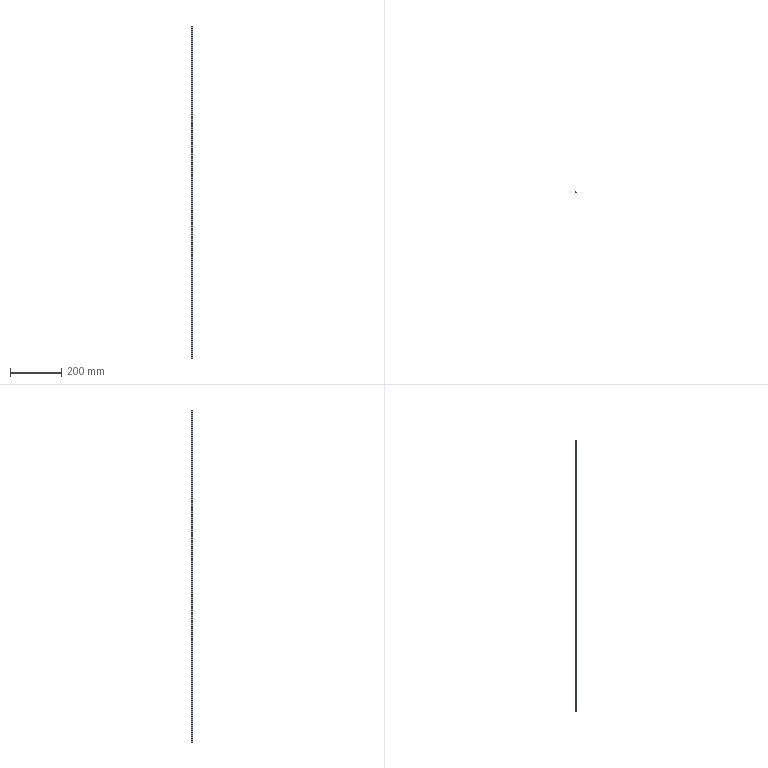Part | SolidWorks | features BaseBody 1 | 1 solid | 6 faces | box 4.859 x 5 x 1300 mm | volume 16237 mm3 | plane 6
STEP:
#1=CARTESIAN_POINT('',(4.859,0.,1300.));
#2=VERTEX_POINT('',#1);
#3=CARTESIAN_POINT('',(4.859,0.1414,1300.));
#4=VERTEX_POINT('',#3);
#5=CARTESIAN_POINT('',(4.859,0.,1300.));
#6=DIRECTION('',(0.,1.,0.));
#7=VECTOR('',#6,1000.);
#8=LINE('',#5,#7);
#9=EDGE_CURVE('',#2,#4,#8,.T.);
#10=ORIENTED_EDGE('',*,*,#9,.F.);
#11=CARTESIAN_POINT('',(4.859,0.,0.));
#12=VERTEX_POINT('',#11);
#13=CARTESIAN_POINT('',(4.859,0.,1300.));
#14=DIRECTION('',(0.,0.,1.));
#15=VECTOR('',#14,1000.);
#16=LINE('',#13,#15);
#17=EDGE_CURVE('',#12,#2,#16,.T.);
#18=ORIENTED_EDGE('',*,*,#17,.F.);
#19=CARTESIAN_POINT('',(4.859,0.1414,0.));
#20=VERTEX_POINT('',#19);
#21=CARTESIAN_POINT('',(4.859,0.1414,0.));
#22=DIRECTION('',(0.,-1.,0.));
#23=VECTOR('',#22,1000.);
#24=LINE('',#21,#23);
#25=EDGE_CURVE('',#20,#12,#24,.T.);
#26=ORIENTED_EDGE('',*,*,#25,.F.);
#27=CARTESIAN_POINT('',(4.859,0.1414,1300.));
#28=DIRECTION('',(0.,0.,-1.));
#29=VECTOR('',#28,1000.);
#30=LINE('',#27,#29);
#31=EDGE_CURVE('',#4,#20,#30,.T.);
#32=ORIENTED_EDGE('',*,*,#31,.F.);
#33=EDGE_LOOP('',(#10,#18,#26,#32));
#34=FACE_OUTER_BOUND('',#33,.T.);
#35=CARTESIAN_POINT('',(4.859,0.1414,1300.));
#36=DIRECTION('',(-1.,0.,0.));
#37=DIRECTION('',(0.,0.,1.));
#38=AXIS2_PLACEMENT_3D('',#35,#36,#37);
#39=PLANE('',#38);
#40=ADVANCED_FACE('',(#34),#39,.F.);
#41=CARTESIAN_POINT('',(0.,5.,0.));
#42=VERTEX_POINT('',#41);
#43=CARTESIAN_POINT('',(5.,0.,0.));
#44=DIRECTION('',(-0.7071,0.7071,0.));
#45=VECTOR('',#44,1000.);
#46=LINE('',#43,#45);
#47=EDGE_CURVE('',#20,#42,#46,.T.);
#48=ORIENTED_EDGE('',*,*,#47,.F.);
#49=ORIENTED_EDGE('',*,*,#25,.T.);
#50=CARTESIAN_POINT('',(0.,0.,0.));
#51=VERTEX_POINT('',#50);
#52=CARTESIAN_POINT('',(0.,0.,0.));
#53=DIRECTION('',(1.,0.,0.));
#54=VECTOR('',#53,1000.);
#55=LINE('',#52,#54);
#56=EDGE_CURVE('',#51,#12,#55,.T.);
#57=ORIENTED_EDGE('',*,*,#56,.F.);
#58=CARTESIAN_POINT('',(0.,0.,0.));
#59=DIRECTION('',(0.,-1.,0.));
#60=VECTOR('',#59,1000.);
#61=LINE('',#58,#60);
#62=EDGE_CURVE('',#42,#51,#61,.T.);
#63=ORIENTED_EDGE('',*,*,#62,.F.);
#64=EDGE_LOOP('',(#48,#49,#57,#63));
#65=FACE_OUTER_BOUND('',#64,.T.);
#66=CARTESIAN_POINT('',(0.,0.,0.));
#67=DIRECTION('',(0.,0.,1.));
#68=DIRECTION('',(1.,0.,0.));
#69=AXIS2_PLACEMENT_3D('',#66,#67,#68);
#70=PLANE('',#69);
#71=ADVANCED_FACE('',(#65),#70,.F.);
#72=CARTESIAN_POINT('',(0.,0.,1300.));
#73=VERTEX_POINT('',#72);
#74=CARTESIAN_POINT('',(0.,0.,1300.));
#75=DIRECTION('',(1.,0.,0.));
#76=VECTOR('',#75,1000.);
#77=LINE('',#74,#76);
#78=EDGE_CURVE('',#73,#2,#77,.T.);
#79=ORIENTED_EDGE('',*,*,#78,.T.);
#80=ORIENTED_EDGE('',*,*,#9,.T.);
#81=CARTESIAN_POINT('',(0.,5.,1300.));
#82=VERTEX_POINT('',#81);
#83=CARTESIAN_POINT('',(5.,0.,1300.));
#84=DIRECTION('',(-0.7071,0.7071,0.));
#85=VECTOR('',#84,1000.);
#86=LINE('',#83,#85);
#87=EDGE_CURVE('',#4,#82,#86,.T.);
#88=ORIENTED_EDGE('',*,*,#87,.T.);
#89=CARTESIAN_POINT('',(0.,0.,1300.));
#90=DIRECTION('',(0.,-1.,0.));
#91=VECTOR('',#90,1000.);
#92=LINE('',#89,#91);
#93=EDGE_CURVE('',#82,#73,#92,.T.);
#94=ORIENTED_EDGE('',*,*,#93,.T.);
#95=EDGE_LOOP('',(#79,#80,#88,#94));
#96=FACE_OUTER_BOUND('',#95,.T.);
#97=CARTESIAN_POINT('',(0.,0.,1300.));
#98=DIRECTION('',(0.,0.,1.));
#99=DIRECTION('',(1.,0.,0.));
#100=AXIS2_PLACEMENT_3D('',#97,#98,#99);
#101=PLANE('',#100);
#102=ADVANCED_FACE('',(#96),#101,.T.);
#103=ORIENTED_EDGE('',*,*,#62,.T.);
#104=CARTESIAN_POINT('',(0.,0.,1300.));
#105=DIRECTION('',(0.,0.,-1.));
#106=VECTOR('',#105,1000.);
#107=LINE('',#104,#106);
#108=EDGE_CURVE('',#73,#51,#107,.T.);
#109=ORIENTED_EDGE('',*,*,#108,.F.);
#110=ORIENTED_EDGE('',*,*,#93,.F.);
#111=CARTESIAN_POINT('',(0.,5.,1300.));
#112=DIRECTION('',(0.,0.,-1.));
#113=VECTOR('',#112,1000.);
#114=LINE('',#111,#113);
#115=EDGE_CURVE('',#82,#42,#114,.T.);
#116=ORIENTED_EDGE('',*,*,#115,.T.);
#117=EDGE_LOOP('',(#103,#109,#110,#116));
#118=FACE_OUTER_BOUND('',#117,.T.);
#119=CARTESIAN_POINT('',(0.,0.,1300.));
#120=DIRECTION('',(1.,0.,0.));
#121=DIRECTION('',(0.,1.,0.));
#122=AXIS2_PLACEMENT_3D('',#119,#120,#121);
#123=PLANE('',#122);
#124=ADVANCED_FACE('',(#118),#123,.F.);
#125=ORIENTED_EDGE('',*,*,#87,.F.);
#126=ORIENTED_EDGE('',*,*,#31,.T.);
#127=ORIENTED_EDGE('',*,*,#47,.T.);
#128=ORIENTED_EDGE('',*,*,#115,.F.);
#129=EDGE_LOOP('',(#125,#126,#127,#128));
#130=FACE_OUTER_BOUND('',#129,.T.);
#131=CARTESIAN_POINT('',(5.,0.,1300.));
#132=DIRECTION('',(-0.7071,-0.7071,0.));
#133=DIRECTION('',(-0.7071,0.7071,0.));
#134=AXIS2_PLACEMENT_3D('',#131,#132,#133);
#135=PLANE('',#134);
#136=ADVANCED_FACE('',(#130),#135,.F.);
#137=ORIENTED_EDGE('',*,*,#56,.T.);
#138=ORIENTED_EDGE('',*,*,#17,.T.);
#139=ORIENTED_EDGE('',*,*,#78,.F.);
#140=ORIENTED_EDGE('',*,*,#108,.T.);
#141=EDGE_LOOP('',(#137,#138,#139,#140));
#142=FACE_OUTER_BOUND('',#141,.T.);
#143=CARTESIAN_POINT('',(0.,0.,1300.));
#144=DIRECTION('',(0.,1.,0.));
#145=DIRECTION('',(1.,0.,0.));
#146=AXIS2_PLACEMENT_3D('',#143,#144,#145);
#147=PLANE('',#146);
#148=ADVANCED_FACE('',(#142),#147,.F.);
#149=CLOSED_SHELL('',(#40,#71,#102,#124,#136,#148));
#150=MANIFOLD_SOLID_BREP('',#149);
#151=CARTESIAN_POINT('',(0.,0.,0.));
#152=DIRECTION('',(0.,0.,1.));
#153=DIRECTION('',(1.,0.,0.));
#154=AXIS2_PLACEMENT_3D('',#151,#152,#153);
#155=(LENGTH_UNIT()NAMED_UNIT(*)SI_UNIT(.MILLI.,.METRE.));
#156=UNCERTAINTY_MEASURE_WITH_UNIT(LENGTH_MEASURE(0.00001),#155,'','');
#157=(NAMED_UNIT(*)PLANE_ANGLE_UNIT()SI_UNIT($,.RADIAN.));
#158=(NAMED_UNIT(*)SI_UNIT($,.STERADIAN.)SOLID_ANGLE_UNIT());
#159=(GEOMETRIC_REPRESENTATION_CONTEXT(3)GLOBAL_UNCERTAINTY_ASSIGNED_CONTEXT((#156))GLOBAL_UNIT_ASSIGNED_CONTEXT((#155,#157,#158))REPRESENTATION_CONTEXT('',''));
#160=ADVANCED_BREP_SHAPE_REPRESENTATION('',(#150,#154),#159);